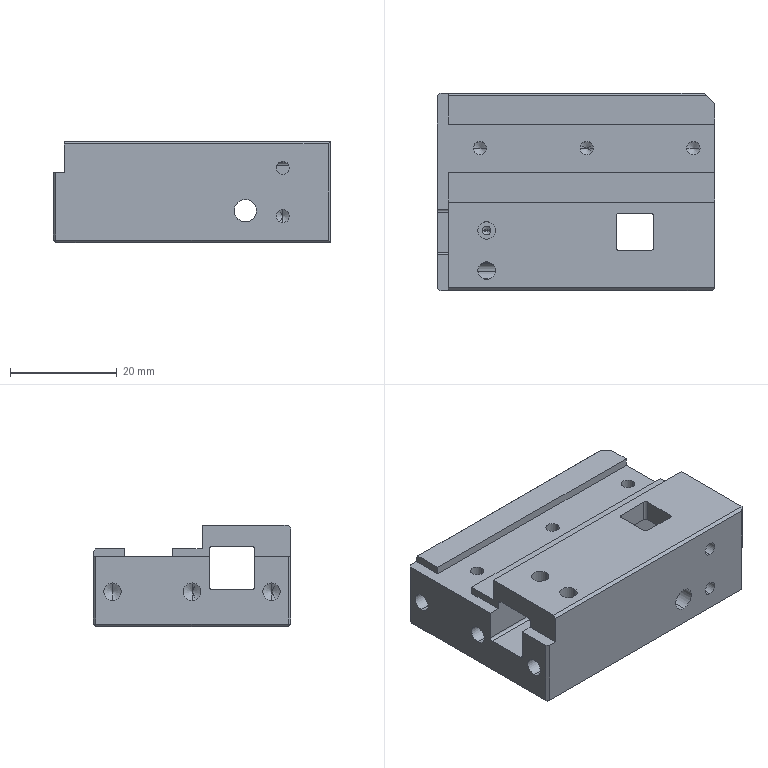Part | SolidWorks | features HoleWzd 8, ICE 8, MoveFace 8, Chamfer 2, Extrusion 1, Fillet 1, MirrorPattern 1, RefAxis 1 | 1 solid | 107 faces | box 52 x 37 x 19 mm | volume 25597 mm3 | cylinder 43 | plane 41 | cone 23 | commonest cylinder face diameters 1 x15 3.3 x14 2.5 x10 4.2 x4